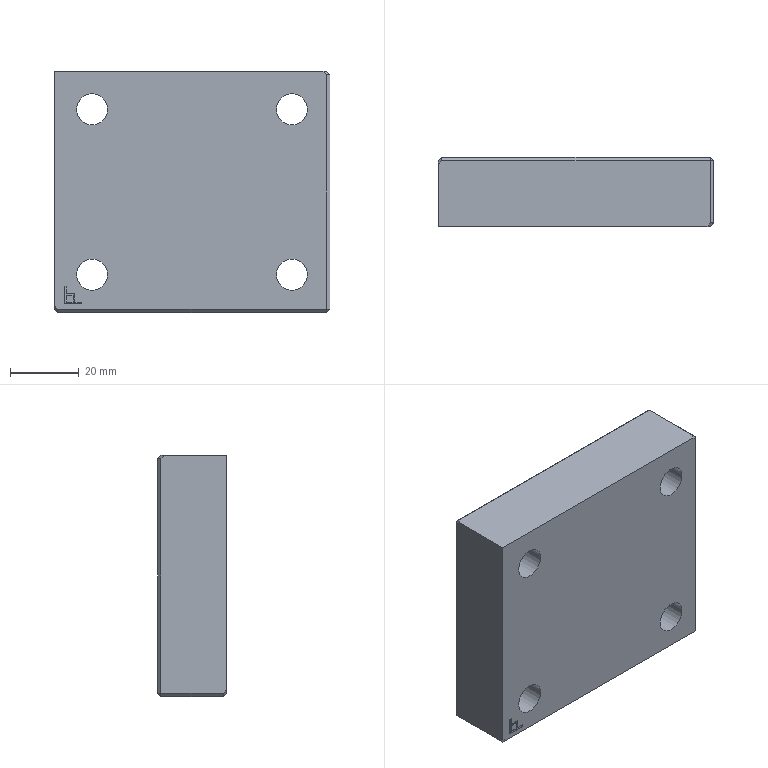Part | SolidWorks | features BaseBody 1 | 1 solid | 56 faces | box 80 x 20 x 70 mm | volume 102134 mm3 | plane 40 | cylinder 16 | commonest cylinder face diameters 9 x8 15 x8
STEP:
#1=CARTESIAN_POINT('',(-353.5,375.,-141.5));
#2=VERTEX_POINT('',#1);
#3=CARTESIAN_POINT('',(-338.5,375.,-141.5));
#4=VERTEX_POINT('',#3);
#5=CARTESIAN_POINT('',(-346.,375.,-141.5));
#6=DIRECTION('',(0.,1.,0.));
#7=DIRECTION('',(-1.,0.,0.));
#8=AXIS2_PLACEMENT_3D('',#5,#6,#7);
#9=CIRCLE('',#8,7.5);
#10=EDGE_CURVE('',#2,#4,#9,.T.);
#11=ORIENTED_EDGE('',*,*,#10,.T.);
#12=CARTESIAN_POINT('',(-338.5,365.,-141.5));
#13=VERTEX_POINT('',#12);
#14=CARTESIAN_POINT('',(-338.5,375.,-141.5));
#15=DIRECTION('',(0.,-1.,0.));
#16=VECTOR('',#15,1000.);
#17=LINE('',#14,#16);
#18=EDGE_CURVE('',#4,#13,#17,.T.);
#19=ORIENTED_EDGE('',*,*,#18,.T.);
#20=CARTESIAN_POINT('',(-353.5,365.,-141.5));
#21=VERTEX_POINT('',#20);
#22=CARTESIAN_POINT('',(-346.,365.,-141.5));
#23=DIRECTION('',(0.,1.,0.));
#24=DIRECTION('',(-1.,0.,0.));
#25=AXIS2_PLACEMENT_3D('',#22,#23,#24);
#26=CIRCLE('',#25,7.5);
#27=EDGE_CURVE('',#21,#13,#26,.T.);
#28=ORIENTED_EDGE('',*,*,#27,.F.);
#29=CARTESIAN_POINT('',(-353.5,375.,-141.5));
#30=DIRECTION('',(0.,-1.,0.));
#31=VECTOR('',#30,1000.);
#32=LINE('',#29,#31);
#33=EDGE_CURVE('',#2,#21,#32,.T.);
#34=ORIENTED_EDGE('',*,*,#33,.F.);
#35=EDGE_LOOP('',(#11,#19,#28,#34));
#36=FACE_OUTER_BOUND('',#35,.T.);
#37=CARTESIAN_POINT('',(-346.,375.,-141.5));
#38=DIRECTION('',(0.,-1.,0.));
#39=DIRECTION('',(-1.,0.,0.));
#40=AXIS2_PLACEMENT_3D('',#37,#38,#39);
#41=CYLINDRICAL_SURFACE('',#40,7.5);
#42=ADVANCED_FACE('',(#36),#41,.F.);
#43=CARTESIAN_POINT('',(-350.5,365.,-141.5));
#44=VERTEX_POINT('',#43);
#45=CARTESIAN_POINT('',(-341.5,365.,-141.5));
#46=VERTEX_POINT('',#45);
#47=CARTESIAN_POINT('',(-346.,365.,-141.5));
#48=DIRECTION('',(0.,1.,0.));
#49=DIRECTION('',(-1.,0.,0.));
#50=AXIS2_PLACEMENT_3D('',#47,#48,#49);
#51=CIRCLE('',#50,4.5);
#52=EDGE_CURVE('',#44,#46,#51,.T.);
#53=ORIENTED_EDGE('',*,*,#52,.T.);
#54=CARTESIAN_POINT('',(-341.5,355.,-141.5));
#55=VERTEX_POINT('',#54);
#56=CARTESIAN_POINT('',(-341.5,325.,-141.5));
#57=DIRECTION('',(0.,-1.,0.));
#58=VECTOR('',#57,1000.);
#59=LINE('',#56,#58);
#60=EDGE_CURVE('',#46,#55,#59,.T.);
#61=ORIENTED_EDGE('',*,*,#60,.T.);
#62=CARTESIAN_POINT('',(-350.5,355.,-141.5));
#63=VERTEX_POINT('',#62);
#64=CARTESIAN_POINT('',(-346.,355.,-141.5));
#65=DIRECTION('',(0.,1.,0.));
#66=DIRECTION('',(-1.,0.,0.));
#67=AXIS2_PLACEMENT_3D('',#64,#65,#66);
#68=CIRCLE('',#67,4.5);
#69=EDGE_CURVE('',#63,#55,#68,.T.);
#70=ORIENTED_EDGE('',*,*,#69,.F.);
#71=CARTESIAN_POINT('',(-350.5,325.,-141.5));
#72=DIRECTION('',(0.,-1.,0.));
#73=VECTOR('',#72,1000.);
#74=LINE('',#71,#73);
#75=EDGE_CURVE('',#44,#63,#74,.T.);
#76=ORIENTED_EDGE('',*,*,#75,.F.);
#77=EDGE_LOOP('',(#53,#61,#70,#76));
#78=FACE_OUTER_BOUND('',#77,.T.);
#79=CARTESIAN_POINT('',(-346.,325.,-141.5));
#80=DIRECTION('',(0.,-1.,0.));
#81=DIRECTION('',(-1.,0.,0.));
#82=AXIS2_PLACEMENT_3D('',#79,#80,#81);
#83=CYLINDRICAL_SURFACE('',#82,4.5);
#84=ADVANCED_FACE('',(#78),#83,.F.);
#85=CARTESIAN_POINT('',(-411.5,375.,-189.5));
#86=VERTEX_POINT('',#85);
#87=CARTESIAN_POINT('',(-396.5,375.,-189.5));
#88=VERTEX_POINT('',#87);
#89=CARTESIAN_POINT('',(-404.,375.,-189.5));
#90=DIRECTION('',(0.,1.,0.));
#91=DIRECTION('',(-1.,0.,0.));
#92=AXIS2_PLACEMENT_3D('',#89,#90,#91);
#93=CIRCLE('',#92,7.5);
#94=EDGE_CURVE('',#86,#88,#93,.T.);
#95=ORIENTED_EDGE('',*,*,#94,.T.);
#96=CARTESIAN_POINT('',(-396.5,365.,-189.5));
#97=VERTEX_POINT('',#96);
#98=CARTESIAN_POINT('',(-396.5,375.,-189.5));
#99=DIRECTION('',(0.,-1.,0.));
#100=VECTOR('',#99,1000.);
#101=LINE('',#98,#100);
#102=EDGE_CURVE('',#88,#97,#101,.T.);
#103=ORIENTED_EDGE('',*,*,#102,.T.);
#104=CARTESIAN_POINT('',(-411.5,365.,-189.5));
#105=VERTEX_POINT('',#104);
#106=CARTESIAN_POINT('',(-404.,365.,-189.5));
#107=DIRECTION('',(0.,1.,0.));
#108=DIRECTION('',(-1.,0.,0.));
#109=AXIS2_PLACEMENT_3D('',#106,#107,#108);
#110=CIRCLE('',#109,7.5);
#111=EDGE_CURVE('',#105,#97,#110,.T.);
#112=ORIENTED_EDGE('',*,*,#111,.F.);
#113=CARTESIAN_POINT('',(-411.5,375.,-189.5));
#114=DIRECTION('',(0.,-1.,0.));
#115=VECTOR('',#114,1000.);
#116=LINE('',#113,#115);
#117=EDGE_CURVE('',#86,#105,#116,.T.);
#118=ORIENTED_EDGE('',*,*,#117,.F.);
#119=EDGE_LOOP('',(#95,#103,#112,#118));
#120=FACE_OUTER_BOUND('',#119,.T.);
#121=CARTESIAN_POINT('',(-404.,375.,-189.5));
#122=DIRECTION('',(0.,-1.,0.));
#123=DIRECTION('',(-1.,0.,0.));
#124=AXIS2_PLACEMENT_3D('',#121,#122,#123);
#125=CYLINDRICAL_SURFACE('',#124,7.5);
#126=ADVANCED_FACE('',(#120),#125,.F.);
#127=CARTESIAN_POINT('',(-408.5,365.,-189.5));
#128=VERTEX_POINT('',#127);
#129=CARTESIAN_POINT('',(-399.5,365.,-189.5));
#130=VERTEX_POINT('',#129);
#131=CARTESIAN_POINT('',(-404.,365.,-189.5));
#132=DIRECTION('',(0.,1.,0.));
#133=DIRECTION('',(-1.,0.,0.));
#134=AXIS2_PLACEMENT_3D('',#131,#132,#133);
#135=CIRCLE('',#134,4.5);
#136=EDGE_CURVE('',#128,#130,#135,.T.);
#137=ORIENTED_EDGE('',*,*,#136,.T.);
#138=CARTESIAN_POINT('',(-399.5,355.,-189.5));
#139=VERTEX_POINT('',#138);
#140=CARTESIAN_POINT('',(-399.5,325.,-189.5));
#141=DIRECTION('',(0.,-1.,0.));
#142=VECTOR('',#141,1000.);
#143=LINE('',#140,#142);
#144=EDGE_CURVE('',#130,#139,#143,.T.);
#145=ORIENTED_EDGE('',*,*,#144,.T.);
#146=CARTESIAN_POINT('',(-408.5,355.,-189.5));
#147=VERTEX_POINT('',#146);
#148=CARTESIAN_POINT('',(-404.,355.,-189.5));
#149=DIRECTION('',(0.,1.,0.));
#150=DIRECTION('',(-1.,0.,0.));
#151=AXIS2_PLACEMENT_3D('',#148,#149,#150);
#152=CIRCLE('',#151,4.5);
#153=EDGE_CURVE('',#147,#139,#152,.T.);
#154=ORIENTED_EDGE('',*,*,#153,.F.);
#155=CARTESIAN_POINT('',(-408.5,325.,-189.5));
#156=DIRECTION('',(0.,-1.,0.));
#157=VECTOR('',#156,1000.);
#158=LINE('',#155,#157);
#159=EDGE_CURVE('',#128,#147,#158,.T.);
#160=ORIENTED_EDGE('',*,*,#159,.F.);
#161=EDGE_LOOP('',(#137,#145,#154,#160));
#162=FACE_OUTER_BOUND('',#161,.T.);
#163=CARTESIAN_POINT('',(-404.,325.,-189.5));
#164=DIRECTION('',(0.,-1.,0.));
#165=DIRECTION('',(-1.,0.,0.));
#166=AXIS2_PLACEMENT_3D('',#163,#164,#165);
#167=CYLINDRICAL_SURFACE('',#166,4.5);
#168=ADVANCED_FACE('',(#162),#167,.F.);
#169=CARTESIAN_POINT('',(-411.5,375.,-141.5));
#170=VERTEX_POINT('',#169);
#171=CARTESIAN_POINT('',(-396.5,375.,-141.5));
#172=VERTEX_POINT('',#171);
#173=CARTESIAN_POINT('',(-404.,375.,-141.5));
#174=DIRECTION('',(0.,1.,0.));
#175=DIRECTION('',(-1.,0.,0.));
#176=AXIS2_PLACEMENT_3D('',#173,#174,#175);
#177=CIRCLE('',#176,7.5);
#178=EDGE_CURVE('',#170,#172,#177,.T.);
#179=ORIENTED_EDGE('',*,*,#178,.T.);
#180=CARTESIAN_POINT('',(-396.5,365.,-141.5));
#181=VERTEX_POINT('',#180);
#182=CARTESIAN_POINT('',(-396.5,375.,-141.5));
#183=DIRECTION('',(0.,-1.,0.));
#184=VECTOR('',#183,1000.);
#185=LINE('',#182,#184);
#186=EDGE_CURVE('',#172,#181,#185,.T.);
#187=ORIENTED_EDGE('',*,*,#186,.T.);
#188=CARTESIAN_POINT('',(-411.5,365.,-141.5));
#189=VERTEX_POINT('',#188);
#190=CARTESIAN_POINT('',(-404.,365.,-141.5));
#191=DIRECTION('',(0.,1.,0.));
#192=DIRECTION('',(-1.,0.,0.));
#193=AXIS2_PLACEMENT_3D('',#190,#191,#192);
#194=CIRCLE('',#193,7.5);
#195=EDGE_CURVE('',#189,#181,#194,.T.);
#196=ORIENTED_EDGE('',*,*,#195,.F.);
#197=CARTESIAN_POINT('',(-411.5,375.,-141.5));
#198=DIRECTION('',(0.,-1.,0.));
#199=VECTOR('',#198,1000.);
#200=LINE('',#197,#199);
#201=EDGE_CURVE('',#170,#189,#200,.T.);
#202=ORIENTED_EDGE('',*,*,#201,.F.);
#203=EDGE_LOOP('',(#179,#187,#196,#202));
#204=FACE_OUTER_BOUND('',#203,.T.);
#205=CARTESIAN_POINT('',(-404.,375.,-141.5));
#206=DIRECTION('',(0.,-1.,0.));
#207=DIRECTION('',(-1.,0.,0.));
#208=AXIS2_PLACEMENT_3D('',#205,#206,#207);
#209=CYLINDRICAL_SURFACE('',#208,7.5);
#210=ADVANCED_FACE('',(#204),#209,.F.);
#211=CARTESIAN_POINT('',(-408.5,365.,-141.5));
#212=VERTEX_POINT('',#211);
#213=CARTESIAN_POINT('',(-399.5,365.,-141.5));
#214=VERTEX_POINT('',#213);
#215=CARTESIAN_POINT('',(-404.,365.,-141.5));
#216=DIRECTION('',(0.,1.,0.));
#217=DIRECTION('',(-1.,0.,0.));
#218=AXIS2_PLACEMENT_3D('',#215,#216,#217);
#219=CIRCLE('',#218,4.5);
#220=EDGE_CURVE('',#212,#214,#219,.T.);
#221=ORIENTED_EDGE('',*,*,#220,.T.);
#222=CARTESIAN_POINT('',(-399.5,355.,-141.5));
#223=VERTEX_POINT('',#222);
#224=CARTESIAN_POINT('',(-399.5,325.,-141.5));
#225=DIRECTION('',(0.,-1.,0.));
#226=VECTOR('',#225,1000.);
#227=LINE('',#224,#226);
#228=EDGE_CURVE('',#214,#223,#227,.T.);
#229=ORIENTED_EDGE('',*,*,#228,.T.);
#230=CARTESIAN_POINT('',(-408.5,355.,-141.5));
#231=VERTEX_POINT('',#230);
#232=CARTESIAN_POINT('',(-404.,355.,-141.5));
#233=DIRECTION('',(0.,1.,0.));
#234=DIRECTION('',(-1.,0.,0.));
#235=AXIS2_PLACEMENT_3D('',#232,#233,#234);
#236=CIRCLE('',#235,4.5);
#237=EDGE_CURVE('',#231,#223,#236,.T.);
#238=ORIENTED_EDGE('',*,*,#237,.F.);
#239=CARTESIAN_POINT('',(-408.5,325.,-141.5));
#240=DIRECTION('',(0.,-1.,0.));
#241=VECTOR('',#240,1000.);
#242=LINE('',#239,#241);
#243=EDGE_CURVE('',#212,#231,#242,.T.);
#244=ORIENTED_EDGE('',*,*,#243,.F.);
#245=EDGE_LOOP('',(#221,#229,#238,#244));
#246=FACE_OUTER_BOUND('',#245,.T.);
#247=CARTESIAN_POINT('',(-404.,325.,-141.5));
#248=DIRECTION('',(0.,-1.,0.));
#249=DIRECTION('',(-1.,0.,0.));
#250=AXIS2_PLACEMENT_3D('',#247,#248,#249);
#251=CYLINDRICAL_SURFACE('',#250,4.5);
#252=ADVANCED_FACE('',(#246),#251,.F.);
#253=CARTESIAN_POINT('',(-353.5,375.,-189.5));
#254=VERTEX_POINT('',#253);
#255=CARTESIAN_POINT('',(-338.5,375.,-189.5));
#256=VERTEX_POINT('',#255);
#257=CARTESIAN_POINT('',(-346.,375.,-189.5));
#258=DIRECTION('',(0.,1.,0.));
#259=DIRECTION('',(-1.,0.,0.));
#260=AXIS2_PLACEMENT_3D('',#257,#258,#259);
#261=CIRCLE('',#260,7.5);
#262=EDGE_CURVE('',#254,#256,#261,.T.);
#263=ORIENTED_EDGE('',*,*,#262,.T.);
#264=CARTESIAN_POINT('',(-338.5,365.,-189.5));
#265=VERTEX_POINT('',#264);
#266=CARTESIAN_POINT('',(-338.5,375.,-189.5));
#267=DIRECTION('',(0.,-1.,0.));
#268=VECTOR('',#267,1000.);
#269=LINE('',#266,#268);
#270=EDGE_CURVE('',#256,#265,#269,.T.);
#271=ORIENTED_EDGE('',*,*,#270,.T.);
#272=CARTESIAN_POINT('',(-353.5,365.,-189.5));
#273=VERTEX_POINT('',#272);
#274=CARTESIAN_POINT('',(-346.,365.,-189.5));
#275=DIRECTION('',(0.,1.,0.));
#276=DIRECTION('',(-1.,0.,0.));
#277=AXIS2_PLACEMENT_3D('',#274,#275,#276);
#278=CIRCLE('',#277,7.5);
#279=EDGE_CURVE('',#273,#265,#278,.T.);
#280=ORIENTED_EDGE('',*,*,#279,.F.);
#281=CARTESIAN_POINT('',(-353.5,375.,-189.5));
#282=DIRECTION('',(0.,-1.,0.));
#283=VECTOR('',#282,1000.);
#284=LINE('',#281,#283);
#285=EDGE_CURVE('',#254,#273,#284,.T.);
#286=ORIENTED_EDGE('',*,*,#285,.F.);
#287=EDGE_LOOP('',(#263,#271,#280,#286));
#288=FACE_OUTER_BOUND('',#287,.T.);
#289=CARTESIAN_POINT('',(-346.,375.,-189.5));
#290=DIRECTION('',(0.,-1.,0.));
#291=DIRECTION('',(-1.,0.,0.));
#292=AXIS2_PLACEMENT_3D('',#289,#290,#291);
#293=CYLINDRICAL_SURFACE('',#292,7.5);
#294=ADVANCED_FACE('',(#288),#293,.F.);
#295=CARTESIAN_POINT('',(-350.5,365.,-189.5));
#296=VERTEX_POINT('',#295);
#297=CARTESIAN_POINT('',(-341.5,365.,-189.5));
#298=VERTEX_POINT('',#297);
#299=CARTESIAN_POINT('',(-346.,365.,-189.5));
#300=DIRECTION('',(0.,1.,0.));
#301=DIRECTION('',(-1.,0.,0.));
#302=AXIS2_PLACEMENT_3D('',#299,#300,#301);
#303=CIRCLE('',#302,4.5);
#304=EDGE_CURVE('',#296,#298,#303,.T.);
#305=ORIENTED_EDGE('',*,*,#304,.T.);
#306=CARTESIAN_POINT('',(-341.5,355.,-189.5));
#307=VERTEX_POINT('',#306);
#308=CARTESIAN_POINT('',(-341.5,325.,-189.5));
#309=DIRECTION('',(0.,-1.,0.));
#310=VECTOR('',#309,1000.);
#311=LINE('',#308,#310);
#312=EDGE_CURVE('',#298,#307,#311,.T.);
#313=ORIENTED_EDGE('',*,*,#312,.T.);
#314=CARTESIAN_POINT('',(-350.5,355.,-189.5));
#315=VERTEX_POINT('',#314);
#316=CARTESIAN_POINT('',(-346.,355.,-189.5));
#317=DIRECTION('',(0.,1.,0.));
#318=DIRECTION('',(-1.,0.,0.));
#319=AXIS2_PLACEMENT_3D('',#316,#317,#318);
#320=CIRCLE('',#319,4.5);
#321=EDGE_CURVE('',#315,#307,#320,.T.);
#322=ORIENTED_EDGE('',*,*,#321,.F.);
#323=CARTESIAN_POINT('',(-350.5,325.,-189.5));
#324=DIRECTION('',(0.,-1.,0.));
#325=VECTOR('',#324,1000.);
#326=LINE('',#323,#325);
#327=EDGE_CURVE('',#296,#315,#326,.T.);
#328=ORIENTED_EDGE('',*,*,#327,.F.);
#329=EDGE_LOOP('',(#305,#313,#322,#328));
#330=FACE_OUTER_BOUND('',#329,.T.);
#331=CARTESIAN_POINT('',(-346.,325.,-189.5));
#332=DIRECTION('',(0.,-1.,0.));
#333=DIRECTION('',(-1.,0.,0.));
#334=AXIS2_PLACEMENT_3D('',#331,#332,#333);
#335=CYLINDRICAL_SURFACE('',#334,4.5);
#336=ADVANCED_FACE('',(#330),#335,.F.);
#337=CARTESIAN_POINT('',(-336.,374.,-130.5));
#338=VERTEX_POINT('',#337);
#339=CARTESIAN_POINT('',(-336.,356.,-130.5));
#340=VERTEX_POINT('',#339);
#341=CARTESIAN_POINT('',(-336.,375.,-130.5));
#342=DIRECTION('',(0.,-1.,0.));
#343=VECTOR('',#342,1000.);
#344=LINE('',#341,#343);
#345=EDGE_CURVE('',#338,#340,#344,.T.);
#346=ORIENTED_EDGE('',*,*,#345,.F.);
#347=CARTESIAN_POINT('',(-414.,374.,-130.5));
#348=VERTEX_POINT('',#347);
#349=CARTESIAN_POINT('',(-333.,374.,-130.5));
#350=DIRECTION('',(1.,0.,0.));
#351=VECTOR('',#350,1000.);
#352=LINE('',#349,#351);
#353=EDGE_CURVE('',#348,#338,#352,.T.);
#354=ORIENTED_EDGE('',*,*,#353,.F.);
#355=CARTESIAN_POINT('',(-415.,373.,-130.5));
#356=VERTEX_POINT('',#355);
#357=CARTESIAN_POINT('',(-373.,415.,-130.5));
#358=DIRECTION('',(-0.7071,-0.7071,0.));
#359=VECTOR('',#358,1000.);
#360=LINE('',#357,#359);
#361=EDGE_CURVE('',#348,#356,#360,.T.);
#362=ORIENTED_EDGE('',*,*,#361,.T.);
#363=CARTESIAN_POINT('',(-415.,355.,-130.5));
#364=VERTEX_POINT('',#363);
#365=CARTESIAN_POINT('',(-415.,354.,-130.5));
#366=DIRECTION('',(0.,1.,0.));
#367=VECTOR('',#366,1000.);
#368=LINE('',#365,#367);
#369=EDGE_CURVE('',#364,#356,#368,.T.);
#370=ORIENTED_EDGE('',*,*,#369,.F.);
#371=CARTESIAN_POINT('',(-337.,355.,-130.5));
#372=VERTEX_POINT('',#371);
#373=CARTESIAN_POINT('',(-333.,355.,-130.5));
#374=DIRECTION('',(1.,0.,0.));
#375=VECTOR('',#374,1000.);
#376=LINE('',#373,#375);
#377=EDGE_CURVE('',#364,#372,#376,.T.);
#378=ORIENTED_EDGE('',*,*,#377,.T.);
#379=CARTESIAN_POINT('',(-336.5,355.5,-130.5));
#380=DIRECTION('',(-0.7071,-0.7071,0.));
#381=VECTOR('',#380,1000.);
#382=LINE('',#379,#381);
#383=EDGE_CURVE('',#340,#372,#382,.T.);
#384=ORIENTED_EDGE('',*,*,#383,.F.);
#385=EDGE_LOOP('',(#346,#354,#362,#370,#378,#384));
#386=FACE_OUTER_BOUND('',#385,.T.);
#387=CARTESIAN_POINT('',(-333.,375.,-130.5));
#388=DIRECTION('',(0.,0.,1.));
#389=DIRECTION('',(-1.,0.,0.));
#390=AXIS2_PLACEMENT_3D('',#387,#388,#389);
#391=PLANE('',#390);
#392=ADVANCED_FACE('',(#386),#391,.T.);
#393=CARTESIAN_POINT('',(-336.,374.,-200.5));
#394=VERTEX_POINT('',#393);
#395=CARTESIAN_POINT('',(-414.,374.,-200.5));
#396=VERTEX_POINT('',#395);
#397=CARTESIAN_POINT('',(-425.,374.,-200.5));
#398=DIRECTION('',(-1.,0.,0.));
#399=VECTOR('',#398,1000.);
#400=LINE('',#397,#399);
#401=EDGE_CURVE('',#394,#396,#400,.T.);
#402=ORIENTED_EDGE('',*,*,#401,.F.);
#403=CARTESIAN_POINT('',(-336.,356.,-200.5));
#404=VERTEX_POINT('',#403);
#405=CARTESIAN_POINT('',(-336.,354.,-200.5));
#406=DIRECTION('',(0.,1.,0.));
#407=VECTOR('',#406,1000.);
#408=LINE('',#405,#407);
#409=EDGE_CURVE('',#404,#394,#408,.T.);
#410=ORIENTED_EDGE('',*,*,#409,.F.);
#411=CARTESIAN_POINT('',(-414.,356.,-200.5));
#412=VERTEX_POINT('',#411);
#413=CARTESIAN_POINT('',(-425.,356.,-200.5));
#414=DIRECTION('',(1.,0.,0.));
#415=VECTOR('',#414,1000.);
#416=LINE('',#413,#415);
#417=EDGE_CURVE('',#412,#404,#416,.T.);
#418=ORIENTED_EDGE('',*,*,#417,.F.);
#419=CARTESIAN_POINT('',(-414.,354.,-200.5));
#420=DIRECTION('',(0.,-1.,0.));
#421=VECTOR('',#420,1000.);
#422=LINE('',#419,#421);
#423=EDGE_CURVE('',#396,#412,#422,.T.);
#424=ORIENTED_EDGE('',*,*,#423,.F.);
#425=EDGE_LOOP('',(#402,#410,#418,#424));
#426=FACE_OUTER_BOUND('',#425,.T.);
#427=CARTESIAN_POINT('',(-425.,354.,-200.5));
#428=DIRECTION('',(0.,0.,-1.));
#429=DIRECTION('',(1.,0.,0.));
#430=AXIS2_PLACEMENT_3D('',#427,#428,#429);
#431=PLANE('',#430);
#432=ADVANCED_FACE('',(#426),#431,.T.);
#433=CARTESIAN_POINT('',(-335.,356.,-199.5));
#434=VERTEX_POINT('',#433);
#435=CARTESIAN_POINT('',(-335.,356.,-131.5));
#436=VERTEX_POINT('',#435);
#437=CARTESIAN_POINT('',(-335.,356.,-18.));
#438=DIRECTION('',(0.,0.,1.));
#439=VECTOR('',#438,1000.);
#440=LINE('',#437,#439);
#441=EDGE_CURVE('',#434,#436,#440,.T.);
#442=ORIENTED_EDGE('',*,*,#441,.F.);
#443=CARTESIAN_POINT('',(-335.,374.,-199.5));
#444=VERTEX_POINT('',#443);
#445=CARTESIAN_POINT('',(-335.,354.,-199.5));
#446=DIRECTION('',(0.,-1.,0.));
#447=VECTOR('',#446,1000.);
#448=LINE('',#445,#447);
#449=EDGE_CURVE('',#444,#434,#448,.T.);
#450=ORIENTED_EDGE('',*,*,#449,.F.);
#451=CARTESIAN_POINT('',(-335.,374.,-131.5));
#452=VERTEX_POINT('',#451);
#453=CARTESIAN_POINT('',(-335.,374.,-18.));
#454=DIRECTION('',(0.,0.,-1.));
#455=VECTOR('',#454,1000.);
#456=LINE('',#453,#455);
#457=EDGE_CURVE('',#452,#444,#456,.T.);
#458=ORIENTED_EDGE('',*,*,#457,.F.);
#459=CARTESIAN_POINT('',(-335.,354.,-131.5));
#460=DIRECTION('',(0.,1.,0.));
#461=VECTOR('',#460,1000.);
#462=LINE('',#459,#461);
#463=EDGE_CURVE('',#436,#452,#462,.T.);
#464=ORIENTED_EDGE('',*,*,#463,.F.);
#465=EDGE_LOOP('',(#442,#450,#458,#464));
#466=FACE_OUTER_BOUND('',#465,.T.);
#467=CARTESIAN_POINT('',(-335.,354.,-18.));
#468=DIRECTION('',(1.,0.,0.));
#469=DIRECTION('',(0.,0.,1.));
#470=AXIS2_PLACEMENT_3D('',#467,#468,#469);
#471=PLANE('',#470);
#472=ADVANCED_FACE('',(#466),#471,.T.);
#473=CARTESIAN_POINT('',(-336.,355.,-131.5));
#474=VERTEX_POINT('',#473);
#475=CARTESIAN_POINT('',(-437.25,355.,-30.25));
#476=DIRECTION('',(-0.7071,0.,0.7071));
#477=VECTOR('',#476,1000.);
#478=LINE('',#475,#477);
#479=EDGE_CURVE('',#474,#372,#478,.T.);
#480=ORIENTED_EDGE('',*,*,#479,.T.);
#481=ORIENTED_EDGE('',*,*,#377,.F.);
#482=CARTESIAN_POINT('',(-415.,355.,-198.5));
#483=VERTEX_POINT('',#482);
#484=CARTESIAN_POINT('',(-415.,355.,-18.));
#485=DIRECTION('',(0.,0.,1.));
#486=VECTOR('',#485,1000.);
#487=LINE('',#484,#486);
#488=EDGE_CURVE('',#483,#364,#487,.T.);
#489=ORIENTED_EDGE('',*,*,#488,.F.);
#490=CARTESIAN_POINT('',(-414.,355.,-199.5));
#491=VERTEX_POINT('',#490);
#492=CARTESIAN_POINT('',(-414.5,355.,-199.));
#493=DIRECTION('',(-0.7071,0.,0.7071));
#494=VECTOR('',#493,1000.);
#495=LINE('',#492,#494);
#496=EDGE_CURVE('',#491,#483,#495,.T.);
#497=ORIENTED_EDGE('',*,*,#496,.F.);
#498=CARTESIAN_POINT('',(-336.,355.,-199.5));
#499=VERTEX_POINT('',#498);
#500=CARTESIAN_POINT('',(-425.,355.,-199.5));
#501=DIRECTION('',(-1.,0.,0.));
#502=VECTOR('',#501,1000.);
#503=LINE('',#500,#502);
#504=EDGE_CURVE('',#499,#491,#503,.T.);
#505=ORIENTED_EDGE('',*,*,#504,.F.);
#506=CARTESIAN_POINT('',(-336.,355.,-18.));
#507=DIRECTION('',(0.,0.,-1.));
#508=VECTOR('',#507,1000.);
#509=LINE('',#506,#508);
#510=EDGE_CURVE('',#474,#499,#509,.T.);
#511=ORIENTED_EDGE('',*,*,#510,.F.);
#512=EDGE_LOOP('',(#480,#481,#489,#497,#505,#511));
#513=FACE_OUTER_BOUND('',#512,.T.);
#514=CARTESIAN_POINT('',(-409.,355.,-195.));
#515=VERTEX_POINT('',#514);
#516=CARTESIAN_POINT('',(-409.,355.,-197.5));
#517=VERTEX_POINT('',#516);
#518=CARTESIAN_POINT('',(-409.,355.,-18.));
#519=DIRECTION('',(0.,0.,-1.));
#520=VECTOR('',#519,1000.);
#521=LINE('',#518,#520);
#522=EDGE_CURVE('',#515,#517,#521,.T.);
#523=ORIENTED_EDGE('',*,*,#522,.T.);
#524=CARTESIAN_POINT('',(-407.,355.,-197.5));
#525=VERTEX_POINT('',#524);
#526=CARTESIAN_POINT('',(-425.,355.,-197.5));
#527=DIRECTION('',(-1.,0.,0.));
#528=VECTOR('',#527,1000.);
#529=LINE('',#526,#528);
#530=EDGE_CURVE('',#525,#517,#529,.T.);
#531=ORIENTED_EDGE('',*,*,#530,.F.);
#532=CARTESIAN_POINT('',(-407.,355.,-198.));
#533=VERTEX_POINT('',#532);
#534=CARTESIAN_POINT('',(-407.,355.,-18.));
#535=DIRECTION('',(0.,0.,-1.));
#536=VECTOR('',#535,1000.);
#537=LINE('',#534,#536);
#538=EDGE_CURVE('',#525,#533,#537,.T.);
#539=ORIENTED_EDGE('',*,*,#538,.T.);
#540=CARTESIAN_POINT('',(-412.,355.,-198.));
#541=VERTEX_POINT('',#540);
#542=CARTESIAN_POINT('',(-425.,355.,-198.));
#543=DIRECTION('',(-1.,0.,0.));
#544=VECTOR('',#543,1000.);
#545=LINE('',#542,#544);
#546=EDGE_CURVE('',#533,#541,#545,.T.);
#547=ORIENTED_EDGE('',*,*,#546,.T.);
#548=CARTESIAN_POINT('',(-412.,355.,-193.));
#549=VERTEX_POINT('',#548);
#550=CARTESIAN_POINT('',(-412.,355.,-18.));
#551=DIRECTION('',(0.,0.,-1.));
#552=VECTOR('',#551,1000.);
#553=LINE('',#550,#552);
#554=EDGE_CURVE('',#549,#541,#553,.T.);
#555=ORIENTED_EDGE('',*,*,#554,.F.);
#556=CARTESIAN_POINT('',(-411.5,355.,-193.));
#557=VERTEX_POINT('',#556);
#558=CARTESIAN_POINT('',(-425.,355.,-193.));
#559=DIRECTION('',(1.,0.,0.));
#560=VECTOR('',#559,1000.);
#561=LINE('',#558,#560);
#562=EDGE_CURVE('',#549,#557,#561,.T.);
#563=ORIENTED_EDGE('',*,*,#562,.T.);
#564=CARTESIAN_POINT('',(-411.5,355.,-195.));
#565=VERTEX_POINT('',#564);
#566=CARTESIAN_POINT('',(-411.5,355.,-18.));
#567=DIRECTION('',(0.,0.,-1.));
#568=VECTOR('',#567,1000.);
#569=LINE('',#566,#568);
#570=EDGE_CURVE('',#557,#565,#569,.T.);
#571=ORIENTED_EDGE('',*,*,#570,.T.);
#572=CARTESIAN_POINT('',(-425.,355.,-195.));
#573=DIRECTION('',(-1.,0.,0.));
#574=VECTOR('',#573,1000.);
#575=LINE('',#572,#574);
#576=EDGE_CURVE('',#515,#565,#575,.T.);
#577=ORIENTED_EDGE('',*,*,#576,.F.);
#578=EDGE_LOOP('',(#523,#531,#539,#547,#555,#563,#571,#577));
#579=FACE_BOUND('',#578,.T.);
#580=ORIENTED_EDGE('',*,*,#69,.T.);
#581=CARTESIAN_POINT('',(-346.,355.,-141.5));
#582=DIRECTION('',(0.,1.,0.));
#583=DIRECTION('',(-1.,0.,0.));
#584=AXIS2_PLACEMENT_3D('',#581,#582,#583);
#585=CIRCLE('',#584,4.5);
#586=EDGE_CURVE('',#55,#63,#585,.T.);
#587=ORIENTED_EDGE('',*,*,#586,.T.);
#588=EDGE_LOOP('',(#580,#587));
#589=FACE_BOUND('',#588,.T.);
#590=ORIENTED_EDGE('',*,*,#153,.T.);
#591=CARTESIAN_POINT('',(-404.,355.,-189.5));
#592=DIRECTION('',(0.,1.,0.));
#593=DIRECTION('',(-1.,0.,0.));
#594=AXIS2_PLACEMENT_3D('',#591,#592,#593);
#595=CIRCLE('',#594,4.5);
#596=EDGE_CURVE('',#139,#147,#595,.T.);
#597=ORIENTED_EDGE('',*,*,#596,.T.);
#598=EDGE_LOOP('',(#590,#597));
#599=FACE_BOUND('',#598,.T.);
#600=ORIENTED_EDGE('',*,*,#237,.T.);
#601=CARTESIAN_POINT('',(-404.,355.,-141.5));
#602=DIRECTION('',(0.,1.,0.));
#603=DIRECTION('',(-1.,0.,0.));
#604=AXIS2_PLACEMENT_3D('',#601,#602,#603);
#605=CIRCLE('',#604,4.5);
#606=EDGE_CURVE('',#223,#231,#605,.T.);
#607=ORIENTED_EDGE('',*,*,#606,.T.);
#608=EDGE_LOOP('',(#600,#607));
#609=FACE_BOUND('',#608,.T.);
#610=ORIENTED_EDGE('',*,*,#321,.T.);
#611=CARTESIAN_POINT('',(-346.,355.,-189.5));
#612=DIRECTION('',(0.,1.,0.));
#613=DIRECTION('',(-1.,0.,0.));
#614=AXIS2_PLACEMENT_3D('',#611,#612,#613);
#615=CIRCLE('',#614,4.5);
#616=EDGE_CURVE('',#307,#315,#615,.T.);
#617=ORIENTED_EDGE('',*,*,#616,.T.);
#618=EDGE_LOOP('',(#610,#617));
#619=FACE_BOUND('',#618,.T.);
#620=CARTESIAN_POINT('',(-425.,355.,-18.));
#621=DIRECTION('',(0.,-1.,0.));
#622=DIRECTION('',(-1.,0.,0.));
#623=AXIS2_PLACEMENT_3D('',#620,#621,#622);
#624=PLANE('',#623);
#625=ADVANCED_FACE('',(#513,#579,#589,#599,#609,#619),#624,.T.);
#626=CARTESIAN_POINT('',(-336.,375.,-199.5));
#627=VERTEX_POINT('',#626);
#628=CARTESIAN_POINT('',(-336.,375.,-131.5));
#629=VERTEX_POINT('',#628);
#630=CARTESIAN_POINT('',(-336.,375.,-18.));
#631=DIRECTION('',(0.,0.,1.));
#632=VECTOR('',#631,1000.);
#633=LINE('',#630,#632);
#634=EDGE_CURVE('',#627,#629,#633,.T.);
#635=ORIENTED_EDGE('',*,*,#634,.F.);
#636=CARTESIAN_POINT('',(-414.,375.,-199.5));
#637=VERTEX_POINT('',#636);
#638=CARTESIAN_POINT('',(-425.,375.,-199.5));
#639=DIRECTION('',(1.,0.,0.));
#640=VECTOR('',#639,1000.);
#641=LINE('',#638,#640);
#642=EDGE_CURVE('',#637,#627,#641,.T.);
#643=ORIENTED_EDGE('',*,*,#642,.F.);
#644=CARTESIAN_POINT('',(-414.,375.,-131.5));
#645=VERTEX_POINT('',#644);
#646=CARTESIAN_POINT('',(-414.,375.,-18.));
#647=DIRECTION('',(0.,0.,-1.));
#648=VECTOR('',#647,1000.);
#649=LINE('',#646,#648);
#650=EDGE_CURVE('',#645,#637,#649,.T.);
#651=ORIENTED_EDGE('',*,*,#650,.F.);
#652=CARTESIAN_POINT('',(-425.,375.,-131.5));
#653=DIRECTION('',(-1.,0.,0.));
#654=VECTOR('',#653,1000.);
#655=LINE('',#652,#654);
#656=EDGE_CURVE('',#629,#645,#655,.T.);
#657=ORIENTED_EDGE('',*,*,#656,.F.);
#658=EDGE_LOOP('',(#635,#643,#651,#657));
#659=FACE_OUTER_BOUND('',#658,.T.);
#660=ORIENTED_EDGE('',*,*,#10,.F.);
#661=CARTESIAN_POINT('',(-346.,375.,-141.5));
#662=DIRECTION('',(0.,1.,0.));
#663=DIRECTION('',(-1.,0.,0.));
#664=AXIS2_PLACEMENT_3D('',#661,#662,#663);
#665=CIRCLE('',#664,7.5);
#666=EDGE_CURVE('',#4,#2,#665,.T.);
#667=ORIENTED_EDGE('',*,*,#666,.F.);
#668=EDGE_LOOP('',(#660,#667));
#669=FACE_BOUND('',#668,.T.);
#670=ORIENTED_EDGE('',*,*,#94,.F.);
#671=CARTESIAN_POINT('',(-404.,375.,-189.5));
#672=DIRECTION('',(0.,1.,0.));
#673=DIRECTION('',(-1.,0.,0.));
#674=AXIS2_PLACEMENT_3D('',#671,#672,#673);
#675=CIRCLE('',#674,7.5);
#676=EDGE_CURVE('',#88,#86,#675,.T.);
#677=ORIENTED_EDGE('',*,*,#676,.F.);
#678=EDGE_LOOP('',(#670,#677));
#679=FACE_BOUND('',#678,.T.);
#680=ORIENTED_EDGE('',*,*,#178,.F.);
#681=CARTESIAN_POINT('',(-404.,375.,-141.5));
#682=DIRECTION('',(0.,1.,0.));
#683=DIRECTION('',(-1.,0.,0.));
#684=AXIS2_PLACEMENT_3D('',#681,#682,#683);
#685=CIRCLE('',#684,7.5);
#686=EDGE_CURVE('',#172,#170,#685,.T.);
#687=ORIENTED_EDGE('',*,*,#686,.F.);
#688=EDGE_LOOP('',(#680,#687));
#689=FACE_BOUND('',#688,.T.);
#690=ORIENTED_EDGE('',*,*,#262,.F.);
#691=CARTESIAN_POINT('',(-346.,375.,-189.5));
#692=DIRECTION('',(0.,1.,0.));
#693=DIRECTION('',(-1.,0.,0.));
#694=AXIS2_PLACEMENT_3D('',#691,#692,#693);
#695=CIRCLE('',#694,7.5);
#696=EDGE_CURVE('',#256,#254,#695,.T.);
#697=ORIENTED_EDGE('',*,*,#696,.F.);
#698=EDGE_LOOP('',(#690,#697));
#699=FACE_BOUND('',#698,.T.);
#700=CARTESIAN_POINT('',(-425.,375.,-18.));
#701=DIRECTION('',(0.,1.,0.));
#702=DIRECTION('',(1.,0.,0.));
#703=AXIS2_PLACEMENT_3D('',#700,#701,#702);
#704=PLANE('',#703);
#705=ADVANCED_FACE('',(#659,#669,#679,#689,#699),#704,.T.);
#706=CARTESIAN_POINT('',(-415.,374.,-199.5));
#707=VERTEX_POINT('',#706);
#708=CARTESIAN_POINT('',(-415.,374.,-131.5));
#709=VERTEX_POINT('',#708);
#710=CARTESIAN_POINT('',(-415.,374.,-18.));
#711=DIRECTION('',(0.,0.,1.));
#712=VECTOR('',#711,1000.);
#713=LINE('',#710,#712);
#714=EDGE_CURVE('',#707,#709,#713,.T.);
#715=ORIENTED_EDGE('',*,*,#714,.F.);
#716=CARTESIAN_POINT('',(-415.,356.,-199.5));
#717=VERTEX_POINT('',#716);
#718=CARTESIAN_POINT('',(-415.,354.,-199.5));
#719=DIRECTION('',(0.,1.,0.));
#720=VECTOR('',#719,1000.);
#721=LINE('',#718,#720);
#722=EDGE_CURVE('',#717,#707,#721,.T.);
#723=ORIENTED_EDGE('',*,*,#722,.F.);
#724=CARTESIAN_POINT('',(-415.,264.25,-107.75));
#725=DIRECTION('',(0.,-0.7071,0.7071));
#726=VECTOR('',#725,1000.);
#727=LINE('',#724,#726);
#728=EDGE_CURVE('',#717,#483,#727,.T.);
#729=ORIENTED_EDGE('',*,*,#728,.T.);
#730=ORIENTED_EDGE('',*,*,#488,.T.);
#731=ORIENTED_EDGE('',*,*,#369,.T.);
#732=CARTESIAN_POINT('',(-415.,373.5,-131.));
#733=DIRECTION('',(0.,-0.7071,0.7071));
#734=VECTOR('',#733,1000.);
#735=LINE('',#732,#734);
#736=EDGE_CURVE('',#709,#356,#735,.T.);
#737=ORIENTED_EDGE('',*,*,#736,.F.);
#738=EDGE_LOOP('',(#715,#723,#729,#730,#731,#737));
#739=FACE_OUTER_BOUND('',#738,.T.);
#740=CARTESIAN_POINT('',(-415.,354.,-18.));
#741=DIRECTION('',(-1.,0.,0.));
#742=DIRECTION('',(0.,0.,-1.));
#743=AXIS2_PLACEMENT_3D('',#740,#741,#742);
#744=PLANE('',#743);
#745=ADVANCED_FACE('',(#739),#744,.T.);
#746=ORIENTED_EDGE('',*,*,#312,.F.);
#747=CARTESIAN_POINT('',(-346.,365.,-189.5));
#748=DIRECTION('',(0.,1.,0.));
#749=DIRECTION('',(-1.,0.,0.));
#750=AXIS2_PLACEMENT_3D('',#747,#748,#749);
#751=CIRCLE('',#750,4.5);
#752=EDGE_CURVE('',#298,#296,#751,.T.);
#753=ORIENTED_EDGE('',*,*,#752,.T.);
#754=ORIENTED_EDGE('',*,*,#327,.T.);
#755=ORIENTED_EDGE('',*,*,#616,.F.);
#756=EDGE_LOOP('',(#746,#753,#754,#755));
#757=FACE_OUTER_BOUND('',#756,.T.);
#758=CARTESIAN_POINT('',(-346.,325.,-189.5));
#759=DIRECTION('',(0.,-1.,0.));
#760=DIRECTION('',(-1.,0.,0.));
#761=AXIS2_PLACEMENT_3D('',#758,#759,#760);
#762=CYLINDRICAL_SURFACE('',#761,4.5);
#763=ADVANCED_FACE('',(#757),#762,.F.);
#764=ORIENTED_EDGE('',*,*,#304,.F.);
#765=ORIENTED_EDGE('',*,*,#752,.F.);
#766=EDGE_LOOP('',(#764,#765));
#767=FACE_BOUND('',#766,.T.);
#768=ORIENTED_EDGE('',*,*,#279,.T.);
#769=CARTESIAN_POINT('',(-346.,365.,-189.5));
#770=DIRECTION('',(0.,1.,0.));
#771=DIRECTION('',(-1.,0.,0.));
#772=AXIS2_PLACEMENT_3D('',#769,#770,#771);
#773=CIRCLE('',#772,7.5);
#774=EDGE_CURVE('',#265,#273,#773,.T.);
#775=ORIENTED_EDGE('',*,*,#774,.T.);
#776=EDGE_LOOP('',(#768,#775));
#777=FACE_OUTER_BOUND('',#776,.T.);
#778=CARTESIAN_POINT('',(-346.,365.,-189.5));
#779=DIRECTION('',(0.,-1.,0.));
#780=DIRECTION('',(-1.,0.,0.));
#781=AXIS2_PLACEMENT_3D('',#778,#779,#780);
#782=PLANE('',#781);
#783=ADVANCED_FACE('',(#767,#777),#782,.F.);
#784=ORIENTED_EDGE('',*,*,#270,.F.);
#785=ORIENTED_EDGE('',*,*,#696,.T.);
#786=ORIENTED_EDGE('',*,*,#285,.T.);
#787=ORIENTED_EDGE('',*,*,#774,.F.);
#788=EDGE_LOOP('',(#784,#785,#786,#787));
#789=FACE_OUTER_BOUND('',#788,.T.);
#790=CARTESIAN_POINT('',(-346.,375.,-189.5));
#791=DIRECTION('',(0.,-1.,0.));
#792=DIRECTION('',(-1.,0.,0.));
#793=AXIS2_PLACEMENT_3D('',#790,#791,#792);
#794=CYLINDRICAL_SURFACE('',#793,7.5);
#795=ADVANCED_FACE('',(#789),#794,.F.);
#796=ORIENTED_EDGE('',*,*,#228,.F.);
#797=CARTESIAN_POINT('',(-404.,365.,-141.5));
#798=DIRECTION('',(0.,1.,0.));
#799=DIRECTION('',(-1.,0.,0.));
#800=AXIS2_PLACEMENT_3D('',#797,#798,#799);
#801=CIRCLE('',#800,4.5);
#802=EDGE_CURVE('',#214,#212,#801,.T.);
#803=ORIENTED_EDGE('',*,*,#802,.T.);
#804=ORIENTED_EDGE('',*,*,#243,.T.);
#805=ORIENTED_EDGE('',*,*,#606,.F.);
#806=EDGE_LOOP('',(#796,#803,#804,#805));
#807=FACE_OUTER_BOUND('',#806,.T.);
#808=CARTESIAN_POINT('',(-404.,325.,-141.5));
#809=DIRECTION('',(0.,-1.,0.));
#810=DIRECTION('',(-1.,0.,0.));
#811=AXIS2_PLACEMENT_3D('',#808,#809,#810);
#812=CYLINDRICAL_SURFACE('',#811,4.5);
#813=ADVANCED_FACE('',(#807),#812,.F.);
#814=ORIENTED_EDGE('',*,*,#220,.F.);
#815=ORIENTED_EDGE('',*,*,#802,.F.);
#816=EDGE_LOOP('',(#814,#815));
#817=FACE_BOUND('',#816,.T.);
#818=ORIENTED_EDGE('',*,*,#195,.T.);
#819=CARTESIAN_POINT('',(-404.,365.,-141.5));
#820=DIRECTION('',(0.,1.,0.));
#821=DIRECTION('',(-1.,0.,0.));
#822=AXIS2_PLACEMENT_3D('',#819,#820,#821);
#823=CIRCLE('',#822,7.5);
#824=EDGE_CURVE('',#181,#189,#823,.T.);
#825=ORIENTED_EDGE('',*,*,#824,.T.);
#826=EDGE_LOOP('',(#818,#825));
#827=FACE_OUTER_BOUND('',#826,.T.);
#828=CARTESIAN_POINT('',(-404.,365.,-141.5));
#829=DIRECTION('',(0.,-1.,0.));
#830=DIRECTION('',(-1.,0.,0.));
#831=AXIS2_PLACEMENT_3D('',#828,#829,#830);
#832=PLANE('',#831);
#833=ADVANCED_FACE('',(#817,#827),#832,.F.);
#834=ORIENTED_EDGE('',*,*,#186,.F.);
#835=ORIENTED_EDGE('',*,*,#686,.T.);
#836=ORIENTED_EDGE('',*,*,#201,.T.);
#837=ORIENTED_EDGE('',*,*,#824,.F.);
#838=EDGE_LOOP('',(#834,#835,#836,#837));
#839=FACE_OUTER_BOUND('',#838,.T.);
#840=CARTESIAN_POINT('',(-404.,375.,-141.5));
#841=DIRECTION('',(0.,-1.,0.));
#842=DIRECTION('',(-1.,0.,0.));
#843=AXIS2_PLACEMENT_3D('',#840,#841,#842);
#844=CYLINDRICAL_SURFACE('',#843,7.5);
#845=ADVANCED_FACE('',(#839),#844,.F.);
#846=ORIENTED_EDGE('',*,*,#144,.F.);
#847=CARTESIAN_POINT('',(-404.,365.,-189.5));
#848=DIRECTION('',(0.,1.,0.));
#849=DIRECTION('',(-1.,0.,0.));
#850=AXIS2_PLACEMENT_3D('',#847,#848,#849);
#851=CIRCLE('',#850,4.5);
#852=EDGE_CURVE('',#130,#128,#851,.T.);
#853=ORIENTED_EDGE('',*,*,#852,.T.);
#854=ORIENTED_EDGE('',*,*,#159,.T.);
#855=ORIENTED_EDGE('',*,*,#596,.F.);
#856=EDGE_LOOP('',(#846,#853,#854,#855));
#857=FACE_OUTER_BOUND('',#856,.T.);
#858=CARTESIAN_POINT('',(-404.,325.,-189.5));
#859=DIRECTION('',(0.,-1.,0.));
#860=DIRECTION('',(-1.,0.,0.));
#861=AXIS2_PLACEMENT_3D('',#858,#859,#860);
#862=CYLINDRICAL_SURFACE('',#861,4.5);
#863=ADVANCED_FACE('',(#857),#862,.F.);
#864=ORIENTED_EDGE('',*,*,#136,.F.);
#865=ORIENTED_EDGE('',*,*,#852,.F.);
#866=EDGE_LOOP('',(#864,#865));
#867=FACE_BOUND('',#866,.T.);
#868=ORIENTED_EDGE('',*,*,#111,.T.);
#869=CARTESIAN_POINT('',(-404.,365.,-189.5));
#870=DIRECTION('',(0.,1.,0.));
#871=DIRECTION('',(-1.,0.,0.));
#872=AXIS2_PLACEMENT_3D('',#869,#870,#871);
#873=CIRCLE('',#872,7.5);
#874=EDGE_CURVE('',#97,#105,#873,.T.);
#875=ORIENTED_EDGE('',*,*,#874,.T.);
#876=EDGE_LOOP('',(#868,#875));
#877=FACE_OUTER_BOUND('',#876,.T.);
#878=CARTESIAN_POINT('',(-404.,365.,-189.5));
#879=DIRECTION('',(0.,-1.,0.));
#880=DIRECTION('',(-1.,0.,0.));
#881=AXIS2_PLACEMENT_3D('',#878,#879,#880);
#882=PLANE('',#881);
#883=ADVANCED_FACE('',(#867,#877),#882,.F.);
#884=ORIENTED_EDGE('',*,*,#102,.F.);
#885=ORIENTED_EDGE('',*,*,#676,.T.);
#886=ORIENTED_EDGE('',*,*,#117,.T.);
#887=ORIENTED_EDGE('',*,*,#874,.F.);
#888=EDGE_LOOP('',(#884,#885,#886,#887));
#889=FACE_OUTER_BOUND('',#888,.T.);
#890=CARTESIAN_POINT('',(-404.,375.,-189.5));
#891=DIRECTION('',(0.,-1.,0.));
#892=DIRECTION('',(-1.,0.,0.));
#893=AXIS2_PLACEMENT_3D('',#890,#891,#892);
#894=CYLINDRICAL_SURFACE('',#893,7.5);
#895=ADVANCED_FACE('',(#889),#894,.F.);
#896=ORIENTED_EDGE('',*,*,#60,.F.);
#897=CARTESIAN_POINT('',(-346.,365.,-141.5));
#898=DIRECTION('',(0.,1.,0.));
#899=DIRECTION('',(-1.,0.,0.));
#900=AXIS2_PLACEMENT_3D('',#897,#898,#899);
#901=CIRCLE('',#900,4.5);
#902=EDGE_CURVE('',#46,#44,#901,.T.);
#903=ORIENTED_EDGE('',*,*,#902,.T.);
#904=ORIENTED_EDGE('',*,*,#75,.T.);
#905=ORIENTED_EDGE('',*,*,#586,.F.);
#906=EDGE_LOOP('',(#896,#903,#904,#905));
#907=FACE_OUTER_BOUND('',#906,.T.);
#908=CARTESIAN_POINT('',(-346.,325.,-141.5));
#909=DIRECTION('',(0.,-1.,0.));
#910=DIRECTION('',(-1.,0.,0.));
#911=AXIS2_PLACEMENT_3D('',#908,#909,#910);
#912=CYLINDRICAL_SURFACE('',#911,4.5);
#913=ADVANCED_FACE('',(#907),#912,.F.);
#914=ORIENTED_EDGE('',*,*,#52,.F.);
#915=ORIENTED_EDGE('',*,*,#902,.F.);
#916=EDGE_LOOP('',(#914,#915));
#917=FACE_BOUND('',#916,.T.);
#918=ORIENTED_EDGE('',*,*,#27,.T.);
#919=CARTESIAN_POINT('',(-346.,365.,-141.5));
#920=DIRECTION('',(0.,1.,0.));
#921=DIRECTION('',(-1.,0.,0.));
#922=AXIS2_PLACEMENT_3D('',#919,#920,#921);
#923=CIRCLE('',#922,7.5);
#924=EDGE_CURVE('',#13,#21,#923,.T.);
#925=ORIENTED_EDGE('',*,*,#924,.T.);
#926=EDGE_LOOP('',(#918,#925));
#927=FACE_OUTER_BOUND('',#926,.T.);
#928=CARTESIAN_POINT('',(-346.,365.,-141.5));
#929=DIRECTION('',(0.,-1.,0.));
#930=DIRECTION('',(-1.,0.,0.));
#931=AXIS2_PLACEMENT_3D('',#928,#929,#930);
#932=PLANE('',#931);
#933=ADVANCED_FACE('',(#917,#927),#932,.F.);
#934=ORIENTED_EDGE('',*,*,#18,.F.);
#935=ORIENTED_EDGE('',*,*,#666,.T.);
#936=ORIENTED_EDGE('',*,*,#33,.T.);
#937=ORIENTED_EDGE('',*,*,#924,.F.);
#938=EDGE_LOOP('',(#934,#935,#936,#937));
#939=FACE_OUTER_BOUND('',#938,.T.);
#940=CARTESIAN_POINT('',(-346.,375.,-141.5));
#941=DIRECTION('',(0.,-1.,0.));
#942=DIRECTION('',(-1.,0.,0.));
#943=AXIS2_PLACEMENT_3D('',#940,#941,#942);
#944=CYLINDRICAL_SURFACE('',#943,7.5);
#945=ADVANCED_FACE('',(#939),#944,.F.);
#946=CARTESIAN_POINT('',(-409.5,355.1,-197.5));
#947=VERTEX_POINT('',#946);
#948=CARTESIAN_POINT('',(-409.5,355.,-197.5));
#949=VERTEX_POINT('',#948);
#950=CARTESIAN_POINT('',(-409.5,355.1,-197.5));
#951=DIRECTION('',(0.,-1.,0.));
#952=VECTOR('',#951,1000.);
#953=LINE('',#950,#952);
#954=EDGE_CURVE('',#947,#949,#953,.T.);
#955=ORIENTED_EDGE('',*,*,#954,.T.);
#956=CARTESIAN_POINT('',(-411.5,355.,-197.5));
#957=VERTEX_POINT('',#956);
#958=CARTESIAN_POINT('',(-425.,355.,-197.5));
#959=DIRECTION('',(-1.,0.,0.));
#960=VECTOR('',#959,1000.);
#961=LINE('',#958,#960);
#962=EDGE_CURVE('',#949,#957,#961,.T.);
#963=ORIENTED_EDGE('',*,*,#962,.T.);
#964=CARTESIAN_POINT('',(-411.5,355.1,-197.5));
#965=VERTEX_POINT('',#964);
#966=CARTESIAN_POINT('',(-411.5,355.1,-197.5));
#967=DIRECTION('',(0.,-1.,0.));
#968=VECTOR('',#967,1000.);
#969=LINE('',#966,#968);
#970=EDGE_CURVE('',#965,#957,#969,.T.);
#971=ORIENTED_EDGE('',*,*,#970,.F.);
#972=CARTESIAN_POINT('',(-411.5,355.1,-197.5));
#973=DIRECTION('',(1.,0.,0.));
#974=VECTOR('',#973,1000.);
#975=LINE('',#972,#974);
#976=EDGE_CURVE('',#965,#947,#975,.T.);
#977=ORIENTED_EDGE('',*,*,#976,.T.);
#978=EDGE_LOOP('',(#955,#963,#971,#977));
#979=FACE_OUTER_BOUND('',#978,.T.);
#980=CARTESIAN_POINT('',(-411.5,355.1,-197.5));
#981=DIRECTION('',(0.,0.,-1.));
#982=DIRECTION('',(0.,1.,0.));
#983=AXIS2_PLACEMENT_3D('',#980,#981,#982);
#984=PLANE('',#983);
#985=ADVANCED_FACE('',(#979),#984,.T.);
#986=CARTESIAN_POINT('',(-411.5,355.,-195.5));
#987=VERTEX_POINT('',#986);
#988=CARTESIAN_POINT('',(-411.5,355.,-18.));
#989=DIRECTION('',(0.,0.,-1.));
#990=VECTOR('',#989,1000.);
#991=LINE('',#988,#990);
#992=EDGE_CURVE('',#987,#957,#991,.T.);
#993=ORIENTED_EDGE('',*,*,#992,.F.);
#994=CARTESIAN_POINT('',(-411.5,355.1,-195.5));
#995=VERTEX_POINT('',#994);
#996=CARTESIAN_POINT('',(-411.5,355.1,-195.5));
#997=DIRECTION('',(0.,-1.,0.));
#998=VECTOR('',#997,1000.);
#999=LINE('',#996,#998);
#1000=EDGE_CURVE('',#995,#987,#999,.T.);
#1001=ORIENTED_EDGE('',*,*,#1000,.F.);
#1002=CARTESIAN_POINT('',(-411.5,355.1,-197.5));
#1003=DIRECTION('',(0.,0.,1.));
#1004=VECTOR('',#1003,1000.);
#1005=LINE('',#1002,#1004);
#1006=EDGE_CURVE('',#965,#995,#1005,.T.);
#1007=ORIENTED_EDGE('',*,*,#1006,.F.);
#1008=ORIENTED_EDGE('',*,*,#970,.T.);
#1009=EDGE_LOOP('',(#993,#1001,#1007,#1008));
#1010=FACE_OUTER_BOUND('',#1009,.T.);
#1011=CARTESIAN_POINT('',(-411.5,355.1,-197.5));
#1012=DIRECTION('',(1.,0.,0.));
#1013=DIRECTION('',(0.,1.,0.));
#1014=AXIS2_PLACEMENT_3D('',#1011,#1012,#1013);
#1015=PLANE('',#1014);
#1016=ADVANCED_FACE('',(#1010),#1015,.F.);
#1017=CARTESIAN_POINT('',(-409.5,355.,-195.5));
#1018=VERTEX_POINT('',#1017);
#1019=CARTESIAN_POINT('',(-425.,355.,-195.5));
#1020=DIRECTION('',(-1.,0.,0.));
#1021=VECTOR('',#1020,1000.);
#1022=LINE('',#1019,#1021);
#1023=EDGE_CURVE('',#1018,#987,#1022,.T.);
#1024=ORIENTED_EDGE('',*,*,#1023,.F.);
#1025=CARTESIAN_POINT('',(-409.5,355.1,-195.5));
#1026=VERTEX_POINT('',#1025);
#1027=CARTESIAN_POINT('',(-409.5,355.1,-195.5));
#1028=DIRECTION('',(0.,-1.,0.));
#1029=VECTOR('',#1028,1000.);
#1030=LINE('',#1027,#1029);
#1031=EDGE_CURVE('',#1026,#1018,#1030,.T.);
#1032=ORIENTED_EDGE('',*,*,#1031,.F.);
#1033=CARTESIAN_POINT('',(-411.5,355.1,-195.5));
#1034=DIRECTION('',(1.,0.,0.));
#1035=VECTOR('',#1034,1000.);
#1036=LINE('',#1033,#1035);
#1037=EDGE_CURVE('',#995,#1026,#1036,.T.);
#1038=ORIENTED_EDGE('',*,*,#1037,.F.);
#1039=ORIENTED_EDGE('',*,*,#1000,.T.);
#1040=EDGE_LOOP('',(#1024,#1032,#1038,#1039));
#1041=FACE_OUTER_BOUND('',#1040,.T.);
#1042=CARTESIAN_POINT('',(-411.5,355.1,-195.5));
#1043=DIRECTION('',(0.,0.,-1.));
#1044=DIRECTION('',(0.,1.,0.));
#1045=AXIS2_PLACEMENT_3D('',#1042,#1043,#1044);
#1046=PLANE('',#1045);
#1047=ADVANCED_FACE('',(#1041),#1046,.F.);
#1048=ORIENTED_EDGE('',*,*,#522,.F.);
#1049=CARTESIAN_POINT('',(-409.,355.1,-195.));
#1050=VERTEX_POINT('',#1049);
#1051=CARTESIAN_POINT('',(-409.,355.1,-195.));
#1052=DIRECTION('',(0.,-1.,0.));
#1053=VECTOR('',#1052,1000.);
#1054=LINE('',#1051,#1053);
#1055=EDGE_CURVE('',#1050,#515,#1054,.T.);
#1056=ORIENTED_EDGE('',*,*,#1055,.F.);
#1057=CARTESIAN_POINT('',(-409.,355.1,-197.5));
#1058=VERTEX_POINT('',#1057);
#1059=CARTESIAN_POINT('',(-409.,355.1,-197.5));
#1060=DIRECTION('',(0.,0.,1.));
#1061=VECTOR('',#1060,1000.);
#1062=LINE('',#1059,#1061);
#1063=EDGE_CURVE('',#1058,#1050,#1062,.T.);
#1064=ORIENTED_EDGE('',*,*,#1063,.F.);
#1065=CARTESIAN_POINT('',(-409.,355.1,-197.5));
#1066=DIRECTION('',(0.,-1.,0.));
#1067=VECTOR('',#1066,1000.);
#1068=LINE('',#1065,#1067);
#1069=EDGE_CURVE('',#1058,#517,#1068,.T.);
#1070=ORIENTED_EDGE('',*,*,#1069,.T.);
#1071=EDGE_LOOP('',(#1048,#1056,#1064,#1070));
#1072=FACE_OUTER_BOUND('',#1071,.T.);
#1073=CARTESIAN_POINT('',(-409.,355.1,-197.5));
#1074=DIRECTION('',(1.,0.,0.));
#1075=DIRECTION('',(0.,1.,0.));
#1076=AXIS2_PLACEMENT_3D('',#1073,#1074,#1075);
#1077=PLANE('',#1076);
#1078=ADVANCED_FACE('',(#1072),#1077,.F.);
#1079=ORIENTED_EDGE('',*,*,#1055,.T.);
#1080=ORIENTED_EDGE('',*,*,#576,.T.);
#1081=CARTESIAN_POINT('',(-411.5,355.1,-195.));
#1082=VERTEX_POINT('',#1081);
#1083=CARTESIAN_POINT('',(-411.5,355.1,-195.));
#1084=DIRECTION('',(0.,-1.,0.));
#1085=VECTOR('',#1084,1000.);
#1086=LINE('',#1083,#1085);
#1087=EDGE_CURVE('',#1082,#565,#1086,.T.);
#1088=ORIENTED_EDGE('',*,*,#1087,.F.);
#1089=CARTESIAN_POINT('',(-411.5,355.1,-195.));
#1090=DIRECTION('',(1.,0.,0.));
#1091=VECTOR('',#1090,1000.);
#1092=LINE('',#1089,#1091);
#1093=EDGE_CURVE('',#1082,#1050,#1092,.T.);
#1094=ORIENTED_EDGE('',*,*,#1093,.T.);
#1095=EDGE_LOOP('',(#1079,#1080,#1088,#1094));
#1096=FACE_OUTER_BOUND('',#1095,.T.);
#1097=CARTESIAN_POINT('',(-411.5,355.1,-195.));
#1098=DIRECTION('',(0.,0.,-1.));
#1099=DIRECTION('',(0.,1.,0.));
#1100=AXIS2_PLACEMENT_3D('',#1097,#1098,#1099);
#1101=PLANE('',#1100);
#1102=ADVANCED_FACE('',(#1096),#1101,.T.);
#1103=ORIENTED_EDGE('',*,*,#570,.F.);
#1104=CARTESIAN_POINT('',(-411.5,355.1,-193.));
#1105=VERTEX_POINT('',#1104);
#1106=CARTESIAN_POINT('',(-411.5,355.1,-193.));
#1107=DIRECTION('',(0.,-1.,0.));
#1108=VECTOR('',#1107,1000.);
#1109=LINE('',#1106,#1108);
#1110=EDGE_CURVE('',#1105,#557,#1109,.T.);
#1111=ORIENTED_EDGE('',*,*,#1110,.F.);
#1112=CARTESIAN_POINT('',(-411.5,355.1,-195.));
#1113=DIRECTION('',(0.,0.,1.));
#1114=VECTOR('',#1113,1000.);
#1115=LINE('',#1112,#1114);
#1116=EDGE_CURVE('',#1082,#1105,#1115,.T.);
#1117=ORIENTED_EDGE('',*,*,#1116,.F.);
#1118=ORIENTED_EDGE('',*,*,#1087,.T.);
#1119=EDGE_LOOP('',(#1103,#1111,#1117,#1118));
#1120=FACE_OUTER_BOUND('',#1119,.T.);
#1121=CARTESIAN_POINT('',(-411.5,355.1,-195.));
#1122=DIRECTION('',(1.,0.,0.));
#1123=DIRECTION('',(0.,1.,0.));
#1124=AXIS2_PLACEMENT_3D('',#1121,#1122,#1123);
#1125=PLANE('',#1124);
#1126=ADVANCED_FACE('',(#1120),#1125,.F.);
#1127=ORIENTED_EDGE('',*,*,#562,.F.);
#1128=CARTESIAN_POINT('',(-412.,355.1,-193.));
#1129=VERTEX_POINT('',#1128);
#1130=CARTESIAN_POINT('',(-412.,355.1,-193.));
#1131=DIRECTION('',(0.,-1.,0.));
#1132=VECTOR('',#1131,1000.);
#1133=LINE('',#1130,#1132);
#1134=EDGE_CURVE('',#1129,#549,#1133,.T.);
#1135=ORIENTED_EDGE('',*,*,#1134,.F.);
#1136=CARTESIAN_POINT('',(-411.5,355.1,-193.));
#1137=DIRECTION('',(-1.,0.,0.));
#1138=VECTOR('',#1137,1000.);
#1139=LINE('',#1136,#1138);
#1140=EDGE_CURVE('',#1105,#1129,#1139,.T.);
#1141=ORIENTED_EDGE('',*,*,#1140,.F.);
#1142=ORIENTED_EDGE('',*,*,#1110,.T.);
#1143=EDGE_LOOP('',(#1127,#1135,#1141,#1142));
#1144=FACE_OUTER_BOUND('',#1143,.T.);
#1145=CARTESIAN_POINT('',(-411.5,355.1,-193.));
#1146=DIRECTION('',(0.,0.,1.));
#1147=DIRECTION('',(0.,-1.,0.));
#1148=AXIS2_PLACEMENT_3D('',#1145,#1146,#1147);
#1149=PLANE('',#1148);
#1150=ADVANCED_FACE('',(#1144),#1149,.F.);
#1151=ORIENTED_EDGE('',*,*,#1134,.T.);
#1152=ORIENTED_EDGE('',*,*,#554,.T.);
#1153=CARTESIAN_POINT('',(-412.,355.1,-198.));
#1154=VERTEX_POINT('',#1153);
#1155=CARTESIAN_POINT('',(-412.,355.1,-198.));
#1156=DIRECTION('',(0.,-1.,0.));
#1157=VECTOR('',#1156,1000.);
#1158=LINE('',#1155,#1157);
#1159=EDGE_CURVE('',#1154,#541,#1158,.T.);
#1160=ORIENTED_EDGE('',*,*,#1159,.F.);
#1161=CARTESIAN_POINT('',(-412.,355.1,-198.));
#1162=DIRECTION('',(0.,0.,1.));
#1163=VECTOR('',#1162,1000.);
#1164=LINE('',#1161,#1163);
#1165=EDGE_CURVE('',#1154,#1129,#1164,.T.);
#1166=ORIENTED_EDGE('',*,*,#1165,.T.);
#1167=EDGE_LOOP('',(#1151,#1152,#1160,#1166));
#1168=FACE_OUTER_BOUND('',#1167,.T.);
#1169=CARTESIAN_POINT('',(-412.,355.1,-198.));
#1170=DIRECTION('',(1.,0.,0.));
#1171=DIRECTION('',(0.,1.,0.));
#1172=AXIS2_PLACEMENT_3D('',#1169,#1170,#1171);
#1173=PLANE('',#1172);
#1174=ADVANCED_FACE('',(#1168),#1173,.T.);
#1175=ORIENTED_EDGE('',*,*,#546,.F.);
#1176=CARTESIAN_POINT('',(-407.,355.1,-198.));
#1177=VERTEX_POINT('',#1176);
#1178=CARTESIAN_POINT('',(-407.,355.1,-198.));
#1179=DIRECTION('',(0.,-1.,0.));
#1180=VECTOR('',#1179,1000.);
#1181=LINE('',#1178,#1180);
#1182=EDGE_CURVE('',#1177,#533,#1181,.T.);
#1183=ORIENTED_EDGE('',*,*,#1182,.F.);
#1184=CARTESIAN_POINT('',(-412.,355.1,-198.));
#1185=DIRECTION('',(1.,0.,0.));
#1186=VECTOR('',#1185,1000.);
#1187=LINE('',#1184,#1186);
#1188=EDGE_CURVE('',#1154,#1177,#1187,.T.);
#1189=ORIENTED_EDGE('',*,*,#1188,.F.);
#1190=ORIENTED_EDGE('',*,*,#1159,.T.);
#1191=EDGE_LOOP('',(#1175,#1183,#1189,#1190));
#1192=FACE_OUTER_BOUND('',#1191,.T.);
#1193=CARTESIAN_POINT('',(-412.,355.1,-198.));
#1194=DIRECTION('',(0.,0.,-1.));
#1195=DIRECTION('',(0.,1.,0.));
#1196=AXIS2_PLACEMENT_3D('',#1193,#1194,#1195);
#1197=PLANE('',#1196);
#1198=ADVANCED_FACE('',(#1192),#1197,.F.);
#1199=ORIENTED_EDGE('',*,*,#538,.F.);
#1200=CARTESIAN_POINT('',(-407.,355.1,-197.5));
#1201=VERTEX_POINT('',#1200);
#1202=CARTESIAN_POINT('',(-407.,355.1,-197.5));
#1203=DIRECTION('',(0.,-1.,0.));
#1204=VECTOR('',#1203,1000.);
#1205=LINE('',#1202,#1204);
#1206=EDGE_CURVE('',#1201,#525,#1205,.T.);
#1207=ORIENTED_EDGE('',*,*,#1206,.F.);
#1208=CARTESIAN_POINT('',(-407.,355.1,-198.));
#1209=DIRECTION('',(0.,0.,1.));
#1210=VECTOR('',#1209,1000.);
#1211=LINE('',#1208,#1210);
#1212=EDGE_CURVE('',#1177,#1201,#1211,.T.);
#1213=ORIENTED_EDGE('',*,*,#1212,.F.);
#1214=ORIENTED_EDGE('',*,*,#1182,.T.);
#1215=EDGE_LOOP('',(#1199,#1207,#1213,#1214));
#1216=FACE_OUTER_BOUND('',#1215,.T.);
#1217=CARTESIAN_POINT('',(-407.,355.1,-198.));
#1218=DIRECTION('',(1.,0.,0.));
#1219=DIRECTION('',(0.,1.,0.));
#1220=AXIS2_PLACEMENT_3D('',#1217,#1218,#1219);
#1221=PLANE('',#1220);
#1222=ADVANCED_FACE('',(#1216),#1221,.F.);
#1223=ORIENTED_EDGE('',*,*,#1206,.T.);
#1224=ORIENTED_EDGE('',*,*,#530,.T.);
#1225=ORIENTED_EDGE('',*,*,#1069,.F.);
#1226=CARTESIAN_POINT('',(-409.,355.1,-197.5));
#1227=DIRECTION('',(1.,0.,0.));
#1228=VECTOR('',#1227,1000.);
#1229=LINE('',#1226,#1228);
#1230=EDGE_CURVE('',#1058,#1201,#1229,.T.);
#1231=ORIENTED_EDGE('',*,*,#1230,.T.);
#1232=EDGE_LOOP('',(#1223,#1224,#1225,#1231));
#1233=FACE_OUTER_BOUND('',#1232,.T.);
#1234=CARTESIAN_POINT('',(-409.,355.1,-197.5));
#1235=DIRECTION('',(0.,0.,-1.));
#1236=DIRECTION('',(0.,1.,0.));
#1237=AXIS2_PLACEMENT_3D('',#1234,#1235,#1236);
#1238=PLANE('',#1237);
#1239=ADVANCED_FACE('',(#1233),#1238,.T.);
#1240=ORIENTED_EDGE('',*,*,#1031,.T.);
#1241=CARTESIAN_POINT('',(-409.5,355.,-18.));
#1242=DIRECTION('',(0.,0.,-1.));
#1243=VECTOR('',#1242,1000.);
#1244=LINE('',#1241,#1243);
#1245=EDGE_CURVE('',#1018,#949,#1244,.T.);
#1246=ORIENTED_EDGE('',*,*,#1245,.T.);
#1247=ORIENTED_EDGE('',*,*,#954,.F.);
#1248=CARTESIAN_POINT('',(-409.5,355.1,-197.5));
#1249=DIRECTION('',(0.,0.,1.));
#1250=VECTOR('',#1249,1000.);
#1251=LINE('',#1248,#1250);
#1252=EDGE_CURVE('',#947,#1026,#1251,.T.);
#1253=ORIENTED_EDGE('',*,*,#1252,.T.);
#1254=EDGE_LOOP('',(#1240,#1246,#1247,#1253));
#1255=FACE_OUTER_BOUND('',#1254,.T.);
#1256=CARTESIAN_POINT('',(-409.5,355.1,-197.5));
#1257=DIRECTION('',(1.,0.,0.));
#1258=DIRECTION('',(0.,1.,0.));
#1259=AXIS2_PLACEMENT_3D('',#1256,#1257,#1258);
#1260=PLANE('',#1259);
#1261=ADVANCED_FACE('',(#1255),#1260,.T.);
#1262=ORIENTED_EDGE('',*,*,#1063,.T.);
#1263=ORIENTED_EDGE('',*,*,#1093,.F.);
#1264=ORIENTED_EDGE('',*,*,#1116,.T.);
#1265=ORIENTED_EDGE('',*,*,#1140,.T.);
#1266=ORIENTED_EDGE('',*,*,#1165,.F.);
#1267=ORIENTED_EDGE('',*,*,#1188,.T.);
#1268=ORIENTED_EDGE('',*,*,#1212,.T.);
#1269=ORIENTED_EDGE('',*,*,#1230,.F.);
#1270=EDGE_LOOP('',(#1262,#1263,#1264,#1265,#1266,#1267,#1268,#1269));
#1271=FACE_OUTER_BOUND('',#1270,.T.);
#1272=ORIENTED_EDGE('',*,*,#976,.F.);
#1273=ORIENTED_EDGE('',*,*,#1006,.T.);
#1274=ORIENTED_EDGE('',*,*,#1037,.T.);
#1275=ORIENTED_EDGE('',*,*,#1252,.F.);
#1276=EDGE_LOOP('',(#1272,#1273,#1274,#1275));
#1277=FACE_BOUND('',#1276,.T.);
#1278=CARTESIAN_POINT('',(-409.,355.1,-195.));
#1279=DIRECTION('',(0.,1.,0.));
#1280=DIRECTION('',(0.,0.,1.));
#1281=AXIS2_PLACEMENT_3D('',#1278,#1279,#1280);
#1282=PLANE('',#1281);
#1283=ADVANCED_FACE('',(#1271,#1277),#1282,.F.);
#1284=ORIENTED_EDGE('',*,*,#1245,.F.);
#1285=ORIENTED_EDGE('',*,*,#1023,.T.);
#1286=ORIENTED_EDGE('',*,*,#992,.T.);
#1287=ORIENTED_EDGE('',*,*,#962,.F.);
#1288=EDGE_LOOP('',(#1284,#1285,#1286,#1287));
#1289=FACE_OUTER_BOUND('',#1288,.T.);
#1290=CARTESIAN_POINT('',(-425.,355.,-18.));
#1291=DIRECTION('',(0.,-1.,0.));
#1292=DIRECTION('',(-1.,0.,0.));
#1293=AXIS2_PLACEMENT_3D('',#1290,#1291,#1292);
#1294=PLANE('',#1293);
#1295=ADVANCED_FACE('',(#1289),#1294,.T.);
#1296=CARTESIAN_POINT('',(-335.,374.,-199.5));
#1297=DIRECTION('',(-0.7071,0.7071,0.));
#1298=VECTOR('',#1297,1000.);
#1299=LINE('',#1296,#1298);
#1300=EDGE_CURVE('',#444,#627,#1299,.T.);
#1301=ORIENTED_EDGE('',*,*,#1300,.T.);
#1302=ORIENTED_EDGE('',*,*,#634,.T.);
#1303=CARTESIAN_POINT('',(-335.5,374.5,-131.5));
#1304=DIRECTION('',(0.7071,-0.7071,0.));
#1305=VECTOR('',#1304,1000.);
#1306=LINE('',#1303,#1305);
#1307=EDGE_CURVE('',#629,#452,#1306,.T.);
#1308=ORIENTED_EDGE('',*,*,#1307,.T.);
#1309=ORIENTED_EDGE('',*,*,#457,.T.);
#1310=EDGE_LOOP('',(#1301,#1302,#1308,#1309));
#1311=FACE_OUTER_BOUND('',#1310,.T.);
#1312=CARTESIAN_POINT('',(-336.,375.,-18.));
#1313=DIRECTION('',(-0.7071,-0.7071,0.));
#1314=DIRECTION('',(-0.7071,0.7071,0.));
#1315=AXIS2_PLACEMENT_3D('',#1312,#1313,#1314);
#1316=PLANE('',#1315);
#1317=ADVANCED_FACE('',(#1311),#1316,.F.);
#1318=CARTESIAN_POINT('',(-335.,374.,-199.5));
#1319=DIRECTION('',(-0.7071,0.,-0.7071));
#1320=VECTOR('',#1319,1000.);
#1321=LINE('',#1318,#1320);
#1322=EDGE_CURVE('',#444,#394,#1321,.T.);
#1323=ORIENTED_EDGE('',*,*,#1322,.T.);
#1324=CARTESIAN_POINT('',(-336.,374.5,-200.));
#1325=DIRECTION('',(0.,0.7071,0.7071));
#1326=VECTOR('',#1325,1000.);
#1327=LINE('',#1324,#1326);
#1328=EDGE_CURVE('',#394,#627,#1327,.T.);
#1329=ORIENTED_EDGE('',*,*,#1328,.T.);
#1330=ORIENTED_EDGE('',*,*,#1300,.F.);
#1331=EDGE_LOOP('',(#1323,#1329,#1330));
#1332=FACE_OUTER_BOUND('',#1331,.T.);
#1333=CARTESIAN_POINT('',(-335.,374.,-199.5));
#1334=DIRECTION('',(0.5774,0.5774,-0.5774));
#1335=DIRECTION('',(0.7071,0.,0.7071));
#1336=AXIS2_PLACEMENT_3D('',#1333,#1334,#1335);
#1337=PLANE('',#1336);
#1338=ADVANCED_FACE('',(#1332),#1337,.T.);
#1339=ORIENTED_EDGE('',*,*,#1307,.F.);
#1340=CARTESIAN_POINT('',(-336.,374.,-130.5));
#1341=DIRECTION('',(0.,-0.7071,0.7071));
#1342=VECTOR('',#1341,1000.);
#1343=LINE('',#1340,#1342);
#1344=EDGE_CURVE('',#629,#338,#1343,.T.);
#1345=ORIENTED_EDGE('',*,*,#1344,.T.);
#1346=CARTESIAN_POINT('',(-336.,374.,-130.5));
#1347=DIRECTION('',(-0.7071,0.,0.7071));
#1348=VECTOR('',#1347,1000.);
#1349=LINE('',#1346,#1348);
#1350=EDGE_CURVE('',#452,#338,#1349,.T.);
#1351=ORIENTED_EDGE('',*,*,#1350,.F.);
#1352=EDGE_LOOP('',(#1339,#1345,#1351));
#1353=FACE_OUTER_BOUND('',#1352,.T.);
#1354=CARTESIAN_POINT('',(-336.,374.,-130.5));
#1355=DIRECTION('',(0.5774,0.5774,0.5774));
#1356=DIRECTION('',(-0.7071,0.,0.7071));
#1357=AXIS2_PLACEMENT_3D('',#1354,#1355,#1356);
#1358=PLANE('',#1357);
#1359=ADVANCED_FACE('',(#1353),#1358,.T.);
#1360=ORIENTED_EDGE('',*,*,#1328,.F.);
#1361=ORIENTED_EDGE('',*,*,#401,.T.);
#1362=CARTESIAN_POINT('',(-414.,375.,-199.5));
#1363=DIRECTION('',(0.,0.7071,0.7071));
#1364=VECTOR('',#1363,1000.);
#1365=LINE('',#1362,#1364);
#1366=EDGE_CURVE('',#396,#637,#1365,.T.);
#1367=ORIENTED_EDGE('',*,*,#1366,.T.);
#1368=ORIENTED_EDGE('',*,*,#642,.T.);
#1369=EDGE_LOOP('',(#1360,#1361,#1367,#1368));
#1370=FACE_OUTER_BOUND('',#1369,.T.);
#1371=CARTESIAN_POINT('',(-425.,375.,-199.5));
#1372=DIRECTION('',(0.,-0.7071,0.7071));
#1373=DIRECTION('',(0.,0.7071,0.7071));
#1374=AXIS2_PLACEMENT_3D('',#1371,#1372,#1373);
#1375=PLANE('',#1374);
#1376=ADVANCED_FACE('',(#1370),#1375,.F.);
#1377=ORIENTED_EDGE('',*,*,#1322,.F.);
#1378=ORIENTED_EDGE('',*,*,#449,.T.);
#1379=CARTESIAN_POINT('',(-336.,356.,-200.5));
#1380=DIRECTION('',(-0.7071,0.,-0.7071));
#1381=VECTOR('',#1380,1000.);
#1382=LINE('',#1379,#1381);
#1383=EDGE_CURVE('',#434,#404,#1382,.T.);
#1384=ORIENTED_EDGE('',*,*,#1383,.T.);
#1385=ORIENTED_EDGE('',*,*,#409,.T.);
#1386=EDGE_LOOP('',(#1377,#1378,#1384,#1385));
#1387=FACE_OUTER_BOUND('',#1386,.T.);
#1388=CARTESIAN_POINT('',(-336.,354.,-200.5));
#1389=DIRECTION('',(-0.7071,0.,0.7071));
#1390=DIRECTION('',(-0.7071,0.,-0.7071));
#1391=AXIS2_PLACEMENT_3D('',#1388,#1389,#1390);
#1392=PLANE('',#1391);
#1393=ADVANCED_FACE('',(#1387),#1392,.F.);
#1394=ORIENTED_EDGE('',*,*,#1344,.F.);
#1395=ORIENTED_EDGE('',*,*,#656,.T.);
#1396=CARTESIAN_POINT('',(-414.,374.,-130.5));
#1397=DIRECTION('',(0.,-0.7071,0.7071));
#1398=VECTOR('',#1397,1000.);
#1399=LINE('',#1396,#1398);
#1400=EDGE_CURVE('',#645,#348,#1399,.T.);
#1401=ORIENTED_EDGE('',*,*,#1400,.T.);
#1402=ORIENTED_EDGE('',*,*,#353,.T.);
#1403=EDGE_LOOP('',(#1394,#1395,#1401,#1402));
#1404=FACE_OUTER_BOUND('',#1403,.T.);
#1405=CARTESIAN_POINT('',(-425.,375.,-131.5));
#1406=DIRECTION('',(0.,-0.7071,-0.7071));
#1407=DIRECTION('',(0.,-0.7071,0.7071));
#1408=AXIS2_PLACEMENT_3D('',#1405,#1406,#1407);
#1409=PLANE('',#1408);
#1410=ADVANCED_FACE('',(#1404),#1409,.F.);
#1411=CARTESIAN_POINT('',(-414.,375.,-199.5));
#1412=DIRECTION('',(-0.7071,-0.7071,0.));
#1413=VECTOR('',#1412,1000.);
#1414=LINE('',#1411,#1413);
#1415=EDGE_CURVE('',#637,#707,#1414,.T.);
#1416=ORIENTED_EDGE('',*,*,#1415,.T.);
#1417=ORIENTED_EDGE('',*,*,#714,.T.);
#1418=CARTESIAN_POINT('',(-414.5,374.5,-131.5));
#1419=DIRECTION('',(0.7071,0.7071,0.));
#1420=VECTOR('',#1419,1000.);
#1421=LINE('',#1418,#1420);
#1422=EDGE_CURVE('',#709,#645,#1421,.T.);
#1423=ORIENTED_EDGE('',*,*,#1422,.T.);
#1424=ORIENTED_EDGE('',*,*,#650,.T.);
#1425=EDGE_LOOP('',(#1416,#1417,#1423,#1424));
#1426=FACE_OUTER_BOUND('',#1425,.T.);
#1427=CARTESIAN_POINT('',(-414.,375.,-18.));
#1428=DIRECTION('',(0.7071,-0.7071,0.));
#1429=DIRECTION('',(-0.7071,-0.7071,0.));
#1430=AXIS2_PLACEMENT_3D('',#1427,#1428,#1429);
#1431=PLANE('',#1430);
#1432=ADVANCED_FACE('',(#1426),#1431,.F.);
#1433=ORIENTED_EDGE('',*,*,#1366,.F.);
#1434=CARTESIAN_POINT('',(-414.5,374.,-200.));
#1435=DIRECTION('',(-0.7071,0.,0.7071));
#1436=VECTOR('',#1435,1000.);
#1437=LINE('',#1434,#1436);
#1438=EDGE_CURVE('',#396,#707,#1437,.T.);
#1439=ORIENTED_EDGE('',*,*,#1438,.T.);
#1440=ORIENTED_EDGE('',*,*,#1415,.F.);
#1441=EDGE_LOOP('',(#1433,#1439,#1440));
#1442=FACE_OUTER_BOUND('',#1441,.T.);
#1443=CARTESIAN_POINT('',(-414.,375.,-199.5));
#1444=DIRECTION('',(-0.5774,0.5774,-0.5774));
#1445=DIRECTION('',(0.7071,0.,-0.7071));
#1446=AXIS2_PLACEMENT_3D('',#1443,#1444,#1445);
#1447=PLANE('',#1446);
#1448=ADVANCED_FACE('',(#1442),#1447,.T.);
#1449=CARTESIAN_POINT('',(-336.,356.,-200.5));
#1450=DIRECTION('',(0.,0.7071,-0.7071));
#1451=VECTOR('',#1450,1000.);
#1452=LINE('',#1449,#1451);
#1453=EDGE_CURVE('',#499,#404,#1452,.T.);
#1454=ORIENTED_EDGE('',*,*,#1453,.T.);
#1455=ORIENTED_EDGE('',*,*,#1383,.F.);
#1456=CARTESIAN_POINT('',(-335.5,355.5,-199.5));
#1457=DIRECTION('',(0.7071,0.7071,0.));
#1458=VECTOR('',#1457,1000.);
#1459=LINE('',#1456,#1458);
#1460=EDGE_CURVE('',#499,#434,#1459,.T.);
#1461=ORIENTED_EDGE('',*,*,#1460,.F.);
#1462=EDGE_LOOP('',(#1454,#1455,#1461));
#1463=FACE_OUTER_BOUND('',#1462,.T.);
#1464=CARTESIAN_POINT('',(-336.,356.,-200.5));
#1465=DIRECTION('',(0.5774,-0.5774,-0.5774));
#1466=DIRECTION('',(0.7071,0.,0.7071));
#1467=AXIS2_PLACEMENT_3D('',#1464,#1465,#1466);
#1468=PLANE('',#1467);
#1469=ADVANCED_FACE('',(#1463),#1468,.T.);
#1470=ORIENTED_EDGE('',*,*,#1422,.F.);
#1471=ORIENTED_EDGE('',*,*,#736,.T.);
#1472=ORIENTED_EDGE('',*,*,#361,.F.);
#1473=ORIENTED_EDGE('',*,*,#1400,.F.);
#1474=EDGE_LOOP('',(#1470,#1471,#1472,#1473));
#1475=FACE_OUTER_BOUND('',#1474,.T.);
#1476=CARTESIAN_POINT('',(-414.,374.,-130.5));
#1477=DIRECTION('',(-0.5774,0.5774,0.5774));
#1478=DIRECTION('',(0.7071,0.7071,0.));
#1479=AXIS2_PLACEMENT_3D('',#1476,#1477,#1478);
#1480=PLANE('',#1479);
#1481=ADVANCED_FACE('',(#1475),#1480,.T.);
#1482=ORIENTED_EDGE('',*,*,#1438,.F.);
#1483=ORIENTED_EDGE('',*,*,#423,.T.);
#1484=CARTESIAN_POINT('',(-415.,356.,-199.5));
#1485=DIRECTION('',(-0.7071,0.,0.7071));
#1486=VECTOR('',#1485,1000.);
#1487=LINE('',#1484,#1486);
#1488=EDGE_CURVE('',#412,#717,#1487,.T.);
#1489=ORIENTED_EDGE('',*,*,#1488,.T.);
#1490=ORIENTED_EDGE('',*,*,#722,.T.);
#1491=EDGE_LOOP('',(#1482,#1483,#1489,#1490));
#1492=FACE_OUTER_BOUND('',#1491,.T.);
#1493=CARTESIAN_POINT('',(-414.,354.,-200.5));
#1494=DIRECTION('',(0.7071,0.,0.7071));
#1495=DIRECTION('',(-0.7071,0.,0.7071));
#1496=AXIS2_PLACEMENT_3D('',#1493,#1494,#1495);
#1497=PLANE('',#1496);
#1498=ADVANCED_FACE('',(#1492),#1497,.F.);
#1499=ORIENTED_EDGE('',*,*,#1453,.F.);
#1500=ORIENTED_EDGE('',*,*,#504,.T.);
#1501=CARTESIAN_POINT('',(-414.,355.5,-200.));
#1502=DIRECTION('',(0.,0.7071,-0.7071));
#1503=VECTOR('',#1502,1000.);
#1504=LINE('',#1501,#1503);
#1505=EDGE_CURVE('',#491,#412,#1504,.T.);
#1506=ORIENTED_EDGE('',*,*,#1505,.T.);
#1507=ORIENTED_EDGE('',*,*,#417,.T.);
#1508=EDGE_LOOP('',(#1499,#1500,#1506,#1507));
#1509=FACE_OUTER_BOUND('',#1508,.T.);
#1510=CARTESIAN_POINT('',(-425.,356.,-200.5));
#1511=DIRECTION('',(0.,0.7071,0.7071));
#1512=DIRECTION('',(0.,0.7071,-0.7071));
#1513=AXIS2_PLACEMENT_3D('',#1510,#1511,#1512);
#1514=PLANE('',#1513);
#1515=ADVANCED_FACE('',(#1509),#1514,.F.);
#1516=ORIENTED_EDGE('',*,*,#1505,.F.);
#1517=ORIENTED_EDGE('',*,*,#496,.T.);
#1518=ORIENTED_EDGE('',*,*,#728,.F.);
#1519=ORIENTED_EDGE('',*,*,#1488,.F.);
#1520=EDGE_LOOP('',(#1516,#1517,#1518,#1519));
#1521=FACE_OUTER_BOUND('',#1520,.T.);
#1522=CARTESIAN_POINT('',(-415.,356.,-199.5));
#1523=DIRECTION('',(-0.5774,-0.5774,-0.5774));
#1524=DIRECTION('',(0.7071,0.,-0.7071));
#1525=AXIS2_PLACEMENT_3D('',#1522,#1523,#1524);
#1526=PLANE('',#1525);
#1527=ADVANCED_FACE('',(#1521),#1526,.T.);
#1528=ORIENTED_EDGE('',*,*,#1460,.T.);
#1529=ORIENTED_EDGE('',*,*,#441,.T.);
#1530=CARTESIAN_POINT('',(-336.,355.,-131.5));
#1531=DIRECTION('',(-0.7071,-0.7071,0.));
#1532=VECTOR('',#1531,1000.);
#1533=LINE('',#1530,#1532);
#1534=EDGE_CURVE('',#436,#474,#1533,.T.);
#1535=ORIENTED_EDGE('',*,*,#1534,.T.);
#1536=ORIENTED_EDGE('',*,*,#510,.T.);
#1537=EDGE_LOOP('',(#1528,#1529,#1535,#1536));
#1538=FACE_OUTER_BOUND('',#1537,.T.);
#1539=CARTESIAN_POINT('',(-336.,355.,-18.));
#1540=DIRECTION('',(-0.7071,0.7071,0.));
#1541=DIRECTION('',(0.7071,0.7071,0.));
#1542=AXIS2_PLACEMENT_3D('',#1539,#1540,#1541);
#1543=PLANE('',#1542);
#1544=ADVANCED_FACE('',(#1538),#1543,.F.);
#1545=ORIENTED_EDGE('',*,*,#1350,.T.);
#1546=ORIENTED_EDGE('',*,*,#345,.T.);
#1547=CARTESIAN_POINT('',(-335.5,356.,-131.));
#1548=DIRECTION('',(0.7071,0.,-0.7071));
#1549=VECTOR('',#1548,1000.);
#1550=LINE('',#1547,#1549);
#1551=EDGE_CURVE('',#340,#436,#1550,.T.);
#1552=ORIENTED_EDGE('',*,*,#1551,.T.);
#1553=ORIENTED_EDGE('',*,*,#463,.T.);
#1554=EDGE_LOOP('',(#1545,#1546,#1552,#1553));
#1555=FACE_OUTER_BOUND('',#1554,.T.);
#1556=CARTESIAN_POINT('',(-335.,354.,-131.5));
#1557=DIRECTION('',(-0.7071,0.,-0.7071));
#1558=DIRECTION('',(0.7071,0.,-0.7071));
#1559=AXIS2_PLACEMENT_3D('',#1556,#1557,#1558);
#1560=PLANE('',#1559);
#1561=ADVANCED_FACE('',(#1555),#1560,.F.);
#1562=ORIENTED_EDGE('',*,*,#1551,.F.);
#1563=ORIENTED_EDGE('',*,*,#383,.T.);
#1564=ORIENTED_EDGE('',*,*,#479,.F.);
#1565=ORIENTED_EDGE('',*,*,#1534,.F.);
#1566=EDGE_LOOP('',(#1562,#1563,#1564,#1565));
#1567=FACE_OUTER_BOUND('',#1566,.T.);
#1568=CARTESIAN_POINT('',(-336.,355.,-131.5));
#1569=DIRECTION('',(0.5774,-0.5774,0.5774));
#1570=DIRECTION('',(-0.7071,0.,0.7071));
#1571=AXIS2_PLACEMENT_3D('',#1568,#1569,#1570);
#1572=PLANE('',#1571);
#1573=ADVANCED_FACE('',(#1567),#1572,.T.);
#1574=CLOSED_SHELL('',(#42,#84,#126,#168,#210,#252,#294,#336,#392,#432,#472,#625,#705,#745,#763,#783,#795,#813,#833,#845,#863,#883,#895,#913,#933,#945,#985,#1016,#1047,#1078,#1102,#1126,#1150,#1174,#1198,#1222,#1239,#1261,#1283,#1295,#1317,#1338,#1359,#1376,#1393,#1410,#1432,#1448,#1469,#1481,#1498,#1515,#1527,#1544,#1561,#1573));
#1575=MANIFOLD_SOLID_BREP('',#1574);
#1576=CARTESIAN_POINT('',(0.,0.,0.));
#1577=DIRECTION('',(0.,0.,1.));
#1578=DIRECTION('',(1.,0.,0.));
#1579=AXIS2_PLACEMENT_3D('',#1576,#1577,#1578);
#1580=(LENGTH_UNIT()NAMED_UNIT(*)SI_UNIT(.MILLI.,.METRE.));
#1581=UNCERTAINTY_MEASURE_WITH_UNIT(LENGTH_MEASURE(0.00001),#1580,'','');
#1582=(NAMED_UNIT(*)PLANE_ANGLE_UNIT()SI_UNIT($,.RADIAN.));
#1583=(NAMED_UNIT(*)SI_UNIT($,.STERADIAN.)SOLID_ANGLE_UNIT());
#1584=(GEOMETRIC_REPRESENTATION_CONTEXT(3)GLOBAL_UNCERTAINTY_ASSIGNED_CONTEXT((#1581))GLOBAL_UNIT_ASSIGNED_CONTEXT((#1580,#1582,#1583))REPRESENTATION_CONTEXT('',''));
#1585=ADVANCED_BREP_SHAPE_REPRESENTATION('',(#1575,#1579),#1584);